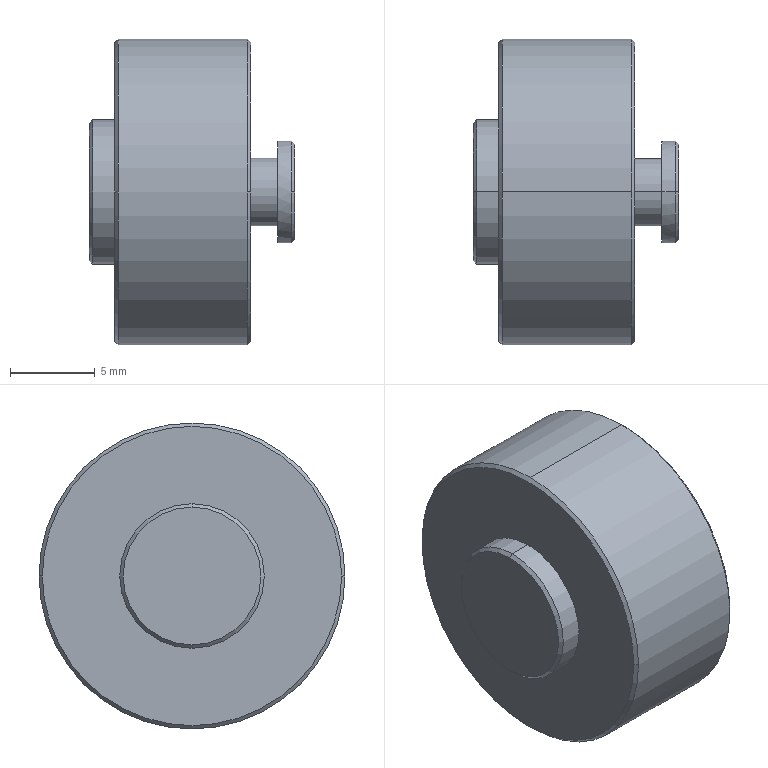Part | STEP file | Guide wheel mechanism revised.sldasm-Part-509 | 1 solid | 22 faces | box 12.1 x 18 x 18 mm | volume 2166 mm3 | cone 9 | cylinder 8 | plane 5 | commonest cylinder face diameters 4 x2 6 x2 8.5 x2 18 x2
STEP:
#1=CARTESIAN_POINT('',(0.,0.,2.));
#2=VERTEX_POINT('',#1);
#3=CARTESIAN_POINT('',(0.,0.,-2.));
#4=VERTEX_POINT('',#3);
#5=CARTESIAN_POINT('',(0.,0.,0.));
#6=DIRECTION('',(-1.,0.,0.));
#7=DIRECTION('',(0.,0.,-1.));
#8=AXIS2_PLACEMENT_3D('',#5,#6,#7);
#9=CIRCLE('',#8,2.);
#10=EDGE_CURVE('',#2,#4,#9,.T.);
#11=ORIENTED_EDGE('',*,*,#10,.F.);
#12=CARTESIAN_POINT('',(1.6,0.,2.));
#13=VERTEX_POINT('',#12);
#14=CARTESIAN_POINT('',(-10.105,0.,2.));
#15=DIRECTION('',(1.,0.,0.));
#16=VECTOR('',#15,1000.);
#17=LINE('',#14,#16);
#18=EDGE_CURVE('',#2,#13,#17,.T.);
#19=ORIENTED_EDGE('',*,*,#18,.T.);
#20=CARTESIAN_POINT('',(1.6,0.,-2.));
#21=VERTEX_POINT('',#20);
#22=CARTESIAN_POINT('',(1.6,0.,0.));
#23=DIRECTION('',(-1.,0.,0.));
#24=DIRECTION('',(0.,0.,-1.));
#25=AXIS2_PLACEMENT_3D('',#22,#23,#24);
#26=CIRCLE('',#25,2.);
#27=EDGE_CURVE('',#13,#21,#26,.T.);
#28=ORIENTED_EDGE('',*,*,#27,.T.);
#29=CARTESIAN_POINT('',(-10.105,0.,-2.));
#30=DIRECTION('',(1.,0.,0.));
#31=VECTOR('',#30,1000.);
#32=LINE('',#29,#31);
#33=EDGE_CURVE('',#4,#21,#32,.T.);
#34=ORIENTED_EDGE('',*,*,#33,.F.);
#35=EDGE_LOOP('',(#11,#19,#28,#34));
#36=FACE_OUTER_BOUND('',#35,.T.);
#37=CARTESIAN_POINT('',(-10.105,0.,0.));
#38=DIRECTION('',(1.,0.,0.));
#39=DIRECTION('',(0.,0.,-1.));
#40=AXIS2_PLACEMENT_3D('',#37,#38,#39);
#41=CYLINDRICAL_SURFACE('',#40,2.);
#42=ADVANCED_FACE('',(#36),#41,.T.);
#43=CARTESIAN_POINT('',(-7.8,9.,0.));
#44=VERTEX_POINT('',#43);
#45=CARTESIAN_POINT('',(-7.8,0.,9.));
#46=VERTEX_POINT('',#45);
#47=CARTESIAN_POINT('',(-7.8,0.,0.));
#48=DIRECTION('',(1.,0.,0.));
#49=DIRECTION('',(0.,0.,-1.));
#50=AXIS2_PLACEMENT_3D('',#47,#48,#49);
#51=CIRCLE('',#50,9.);
#52=EDGE_CURVE('',#44,#46,#51,.T.);
#53=ORIENTED_EDGE('',*,*,#52,.T.);
#54=CARTESIAN_POINT('',(-0.2,0.,9.));
#55=VERTEX_POINT('',#54);
#56=CARTESIAN_POINT('',(-10.105,0.,9.));
#57=DIRECTION('',(1.,0.,0.));
#58=VECTOR('',#57,1000.);
#59=LINE('',#56,#58);
#60=EDGE_CURVE('',#46,#55,#59,.T.);
#61=ORIENTED_EDGE('',*,*,#60,.T.);
#62=CARTESIAN_POINT('',(-0.2,9.,0.));
#63=VERTEX_POINT('',#62);
#64=CARTESIAN_POINT('',(-0.2,0.,0.));
#65=DIRECTION('',(1.,0.,0.));
#66=DIRECTION('',(0.,0.,-1.));
#67=AXIS2_PLACEMENT_3D('',#64,#65,#66);
#68=CIRCLE('',#67,9.);
#69=EDGE_CURVE('',#63,#55,#68,.T.);
#70=ORIENTED_EDGE('',*,*,#69,.F.);
#71=CARTESIAN_POINT('',(-0.2,0.,-9.));
#72=VERTEX_POINT('',#71);
#73=CARTESIAN_POINT('',(-0.2,0.,0.));
#74=DIRECTION('',(1.,0.,0.));
#75=DIRECTION('',(0.,0.,-1.));
#76=AXIS2_PLACEMENT_3D('',#73,#74,#75);
#77=CIRCLE('',#76,9.);
#78=EDGE_CURVE('',#72,#63,#77,.T.);
#79=ORIENTED_EDGE('',*,*,#78,.F.);
#80=CARTESIAN_POINT('',(-7.8,0.,-9.));
#81=VERTEX_POINT('',#80);
#82=CARTESIAN_POINT('',(-10.105,0.,-9.));
#83=DIRECTION('',(1.,0.,0.));
#84=VECTOR('',#83,1000.);
#85=LINE('',#82,#84);
#86=EDGE_CURVE('',#81,#72,#85,.T.);
#87=ORIENTED_EDGE('',*,*,#86,.F.);
#88=CARTESIAN_POINT('',(-7.8,0.,0.));
#89=DIRECTION('',(1.,0.,0.));
#90=DIRECTION('',(0.,0.,-1.));
#91=AXIS2_PLACEMENT_3D('',#88,#89,#90);
#92=CIRCLE('',#91,9.);
#93=EDGE_CURVE('',#81,#44,#92,.T.);
#94=ORIENTED_EDGE('',*,*,#93,.T.);
#95=EDGE_LOOP('',(#53,#61,#70,#79,#87,#94));
#96=FACE_OUTER_BOUND('',#95,.T.);
#97=CARTESIAN_POINT('',(-10.105,0.,0.));
#98=DIRECTION('',(1.,0.,0.));
#99=DIRECTION('',(0.,0.,-1.));
#100=AXIS2_PLACEMENT_3D('',#97,#98,#99);
#101=CYLINDRICAL_SURFACE('',#100,9.);
#102=ADVANCED_FACE('',(#96),#101,.T.);
#103=CARTESIAN_POINT('',(1.6,0.,-3.));
#104=VERTEX_POINT('',#103);
#105=CARTESIAN_POINT('',(1.6,0.,3.));
#106=VERTEX_POINT('',#105);
#107=CARTESIAN_POINT('',(1.6,0.,0.));
#108=DIRECTION('',(1.,0.,0.));
#109=DIRECTION('',(0.,0.,-1.));
#110=AXIS2_PLACEMENT_3D('',#107,#108,#109);
#111=CIRCLE('',#110,3.);
#112=EDGE_CURVE('',#104,#106,#111,.T.);
#113=ORIENTED_EDGE('',*,*,#112,.T.);
#114=CARTESIAN_POINT('',(2.4,0.,3.));
#115=VERTEX_POINT('',#114);
#116=CARTESIAN_POINT('',(-10.105,0.,3.));
#117=DIRECTION('',(1.,0.,0.));
#118=VECTOR('',#117,1000.);
#119=LINE('',#116,#118);
#120=EDGE_CURVE('',#106,#115,#119,.T.);
#121=ORIENTED_EDGE('',*,*,#120,.T.);
#122=CARTESIAN_POINT('',(2.4,3.,0.));
#123=VERTEX_POINT('',#122);
#124=CARTESIAN_POINT('',(2.4,0.,0.));
#125=DIRECTION('',(-1.,0.,0.));
#126=DIRECTION('',(0.,0.,-1.));
#127=AXIS2_PLACEMENT_3D('',#124,#125,#126);
#128=CIRCLE('',#127,3.);
#129=EDGE_CURVE('',#115,#123,#128,.T.);
#130=ORIENTED_EDGE('',*,*,#129,.T.);
#131=CARTESIAN_POINT('',(2.4,0.,-3.));
#132=VERTEX_POINT('',#131);
#133=CARTESIAN_POINT('',(2.4,0.,0.));
#134=DIRECTION('',(-1.,0.,0.));
#135=DIRECTION('',(0.,0.,-1.));
#136=AXIS2_PLACEMENT_3D('',#133,#134,#135);
#137=CIRCLE('',#136,3.);
#138=EDGE_CURVE('',#123,#132,#137,.T.);
#139=ORIENTED_EDGE('',*,*,#138,.T.);
#140=CARTESIAN_POINT('',(-10.105,0.,-3.));
#141=DIRECTION('',(1.,0.,0.));
#142=VECTOR('',#141,1000.);
#143=LINE('',#140,#142);
#144=EDGE_CURVE('',#104,#132,#143,.T.);
#145=ORIENTED_EDGE('',*,*,#144,.F.);
#146=EDGE_LOOP('',(#113,#121,#130,#139,#145));
#147=FACE_OUTER_BOUND('',#146,.T.);
#148=CARTESIAN_POINT('',(-10.105,0.,0.));
#149=DIRECTION('',(1.,0.,0.));
#150=DIRECTION('',(0.,0.,-1.));
#151=AXIS2_PLACEMENT_3D('',#148,#149,#150);
#152=CYLINDRICAL_SURFACE('',#151,3.);
#153=ADVANCED_FACE('',(#147),#152,.T.);
#154=CARTESIAN_POINT('',(2.6,-2.8,0.));
#155=VERTEX_POINT('',#154);
#156=CARTESIAN_POINT('',(2.6,0.,2.8));
#157=VERTEX_POINT('',#156);
#158=CARTESIAN_POINT('',(2.6,0.,0.));
#159=DIRECTION('',(-1.,0.,0.));
#160=DIRECTION('',(0.,0.,1.));
#161=AXIS2_PLACEMENT_3D('',#158,#159,#160);
#162=CIRCLE('',#161,2.8);
#163=EDGE_CURVE('',#155,#157,#162,.T.);
#164=ORIENTED_EDGE('',*,*,#163,.T.);
#165=CARTESIAN_POINT('',(2.4,0.,3.));
#166=DIRECTION('',(-0.7071,0.,0.7071));
#167=VECTOR('',#166,1000.);
#168=LINE('',#165,#167);
#169=EDGE_CURVE('',#157,#115,#168,.T.);
#170=ORIENTED_EDGE('',*,*,#169,.T.);
#171=CARTESIAN_POINT('',(2.4,-3.,0.));
#172=VERTEX_POINT('',#171);
#173=CARTESIAN_POINT('',(2.4,0.,0.));
#174=DIRECTION('',(-1.,0.,0.));
#175=DIRECTION('',(0.,0.,-1.));
#176=AXIS2_PLACEMENT_3D('',#173,#174,#175);
#177=CIRCLE('',#176,3.);
#178=EDGE_CURVE('',#172,#115,#177,.T.);
#179=ORIENTED_EDGE('',*,*,#178,.F.);
#180=CARTESIAN_POINT('',(-498994.601,-499000.,0.000000194));
#181=DIRECTION('',(-0.7071,-0.7071,0.));
#182=VECTOR('',#181,1000.);
#183=LINE('',#180,#182);
#184=EDGE_CURVE('',#155,#172,#183,.T.);
#185=ORIENTED_EDGE('',*,*,#184,.F.);
#186=EDGE_LOOP('',(#164,#170,#179,#185));
#187=FACE_OUTER_BOUND('',#186,.T.);
#188=CARTESIAN_POINT('',(2.4,0.,0.));
#189=DIRECTION('',(-1.,0.,0.));
#190=DIRECTION('',(0.,0.,1.));
#191=AXIS2_PLACEMENT_3D('',#188,#189,#190);
#192=CONICAL_SURFACE('',#191,3.,0.7854);
#193=ADVANCED_FACE('',(#187),#192,.T.);
#194=CARTESIAN_POINT('',(-9.3,0.,-4.25));
#195=VERTEX_POINT('',#194);
#196=CARTESIAN_POINT('',(-9.3,0.,4.25));
#197=VERTEX_POINT('',#196);
#198=CARTESIAN_POINT('',(-9.3,0.,0.));
#199=DIRECTION('',(1.,0.,0.));
#200=DIRECTION('',(0.,0.,-1.));
#201=AXIS2_PLACEMENT_3D('',#198,#199,#200);
#202=CIRCLE('',#201,4.25);
#203=EDGE_CURVE('',#195,#197,#202,.T.);
#204=ORIENTED_EDGE('',*,*,#203,.T.);
#205=CARTESIAN_POINT('',(-8.,0.,4.25));
#206=VERTEX_POINT('',#205);
#207=CARTESIAN_POINT('',(-10.105,0.,4.25));
#208=DIRECTION('',(1.,0.,0.));
#209=VECTOR('',#208,1000.);
#210=LINE('',#207,#209);
#211=EDGE_CURVE('',#197,#206,#210,.T.);
#212=ORIENTED_EDGE('',*,*,#211,.T.);
#213=CARTESIAN_POINT('',(-8.,0.,-4.25));
#214=VERTEX_POINT('',#213);
#215=CARTESIAN_POINT('',(-8.,0.,0.));
#216=DIRECTION('',(-1.,0.,0.));
#217=DIRECTION('',(0.,0.,-1.));
#218=AXIS2_PLACEMENT_3D('',#215,#216,#217);
#219=CIRCLE('',#218,4.25);
#220=EDGE_CURVE('',#206,#214,#219,.T.);
#221=ORIENTED_EDGE('',*,*,#220,.T.);
#222=CARTESIAN_POINT('',(-10.105,0.,-4.25));
#223=DIRECTION('',(1.,0.,0.));
#224=VECTOR('',#223,1000.);
#225=LINE('',#222,#224);
#226=EDGE_CURVE('',#195,#214,#225,.T.);
#227=ORIENTED_EDGE('',*,*,#226,.F.);
#228=EDGE_LOOP('',(#204,#212,#221,#227));
#229=FACE_OUTER_BOUND('',#228,.T.);
#230=CARTESIAN_POINT('',(-10.105,0.,0.));
#231=DIRECTION('',(1.,0.,0.));
#232=DIRECTION('',(0.,0.,-1.));
#233=AXIS2_PLACEMENT_3D('',#230,#231,#232);
#234=CYLINDRICAL_SURFACE('',#233,4.25);
#235=ADVANCED_FACE('',(#229),#234,.T.);
#236=CARTESIAN_POINT('',(-9.5,0.,-4.05));
#237=VERTEX_POINT('',#236);
#238=CARTESIAN_POINT('',(-9.5,0.,4.05));
#239=VERTEX_POINT('',#238);
#240=CARTESIAN_POINT('',(-9.5,0.,0.));
#241=DIRECTION('',(1.,0.,0.));
#242=DIRECTION('',(0.,0.,-1.));
#243=AXIS2_PLACEMENT_3D('',#240,#241,#242);
#244=CIRCLE('',#243,4.05);
#245=EDGE_CURVE('',#237,#239,#244,.T.);
#246=ORIENTED_EDGE('',*,*,#245,.T.);
#247=CARTESIAN_POINT('',(-9.3,0.,4.25));
#248=DIRECTION('',(0.7071,0.,0.7071));
#249=VECTOR('',#248,1000.);
#250=LINE('',#247,#249);
#251=EDGE_CURVE('',#239,#197,#250,.T.);
#252=ORIENTED_EDGE('',*,*,#251,.T.);
#253=ORIENTED_EDGE('',*,*,#203,.F.);
#254=CARTESIAN_POINT('',(-9.3,0.,-4.25));
#255=DIRECTION('',(0.7071,0.,-0.7071));
#256=VECTOR('',#255,1000.);
#257=LINE('',#254,#256);
#258=EDGE_CURVE('',#237,#195,#257,.T.);
#259=ORIENTED_EDGE('',*,*,#258,.F.);
#260=EDGE_LOOP('',(#246,#252,#253,#259));
#261=FACE_OUTER_BOUND('',#260,.T.);
#262=CARTESIAN_POINT('',(-9.3,0.,0.));
#263=DIRECTION('',(1.,0.,0.));
#264=DIRECTION('',(0.,0.,-1.));
#265=AXIS2_PLACEMENT_3D('',#262,#263,#264);
#266=CONICAL_SURFACE('',#265,4.25,0.7854);
#267=ADVANCED_FACE('',(#261),#266,.T.);
#268=CARTESIAN_POINT('',(0.,0.,0.));
#269=DIRECTION('',(-1.,0.,0.));
#270=DIRECTION('',(0.,0.,-1.));
#271=AXIS2_PLACEMENT_3D('',#268,#269,#270);
#272=CIRCLE('',#271,2.);
#273=EDGE_CURVE('',#4,#2,#272,.T.);
#274=ORIENTED_EDGE('',*,*,#273,.T.);
#275=ORIENTED_EDGE('',*,*,#10,.T.);
#276=EDGE_LOOP('',(#274,#275));
#277=FACE_BOUND('',#276,.T.);
#278=CARTESIAN_POINT('',(-0.000000022,8.8,0.));
#279=VERTEX_POINT('',#278);
#280=CARTESIAN_POINT('',(-0.000000022,-8.8,0.));
#281=VERTEX_POINT('',#280);
#282=CARTESIAN_POINT('',(-0.000000022,0.,0.));
#283=DIRECTION('',(1.,0.,0.));
#284=DIRECTION('',(0.,-1.,0.));
#285=AXIS2_PLACEMENT_3D('',#282,#283,#284);
#286=CIRCLE('',#285,8.8);
#287=EDGE_CURVE('',#279,#281,#286,.T.);
#288=ORIENTED_EDGE('',*,*,#287,.T.);
#289=CARTESIAN_POINT('',(-0.000000022,0.,0.));
#290=DIRECTION('',(1.,0.,0.));
#291=DIRECTION('',(0.,0.,1.));
#292=AXIS2_PLACEMENT_3D('',#289,#290,#291);
#293=CIRCLE('',#292,8.8);
#294=EDGE_CURVE('',#281,#279,#293,.T.);
#295=ORIENTED_EDGE('',*,*,#294,.T.);
#296=EDGE_LOOP('',(#288,#295));
#297=FACE_OUTER_BOUND('',#296,.T.);
#298=CARTESIAN_POINT('',(0.,0.,0.));
#299=DIRECTION('',(1.,0.,0.));
#300=DIRECTION('',(0.,0.,-1.));
#301=AXIS2_PLACEMENT_3D('',#298,#299,#300);
#302=PLANE('',#301);
#303=ADVANCED_FACE('',(#277,#297),#302,.T.);
#304=ORIENTED_EDGE('',*,*,#18,.F.);
#305=ORIENTED_EDGE('',*,*,#273,.F.);
#306=ORIENTED_EDGE('',*,*,#33,.T.);
#307=CARTESIAN_POINT('',(1.6,0.,0.));
#308=DIRECTION('',(-1.,0.,0.));
#309=DIRECTION('',(0.,0.,-1.));
#310=AXIS2_PLACEMENT_3D('',#307,#308,#309);
#311=CIRCLE('',#310,2.);
#312=EDGE_CURVE('',#21,#13,#311,.T.);
#313=ORIENTED_EDGE('',*,*,#312,.T.);
#314=EDGE_LOOP('',(#304,#305,#306,#313));
#315=FACE_OUTER_BOUND('',#314,.T.);
#316=CARTESIAN_POINT('',(-10.105,0.,0.));
#317=DIRECTION('',(1.,0.,0.));
#318=DIRECTION('',(0.,0.,-1.));
#319=AXIS2_PLACEMENT_3D('',#316,#317,#318);
#320=CYLINDRICAL_SURFACE('',#319,2.);
#321=ADVANCED_FACE('',(#315),#320,.T.);
#322=CARTESIAN_POINT('',(-0.2,-9.,0.));
#323=VERTEX_POINT('',#322);
#324=CARTESIAN_POINT('',(-498991.203,-499000.,0.000000013));
#325=DIRECTION('',(-0.7071,-0.7071,0.));
#326=VECTOR('',#325,1000.);
#327=LINE('',#324,#326);
#328=EDGE_CURVE('',#281,#323,#327,.T.);
#329=ORIENTED_EDGE('',*,*,#328,.T.);
#330=CARTESIAN_POINT('',(-0.2,0.,0.));
#331=DIRECTION('',(1.,0.,0.));
#332=DIRECTION('',(0.,0.,-1.));
#333=AXIS2_PLACEMENT_3D('',#330,#331,#332);
#334=CIRCLE('',#333,9.);
#335=EDGE_CURVE('',#323,#72,#334,.T.);
#336=ORIENTED_EDGE('',*,*,#335,.T.);
#337=ORIENTED_EDGE('',*,*,#78,.T.);
#338=CARTESIAN_POINT('',(-498991.203,499000.,0.000000012));
#339=DIRECTION('',(0.7071,-0.7071,0.));
#340=VECTOR('',#339,1000.);
#341=LINE('',#338,#340);
#342=EDGE_CURVE('',#63,#279,#341,.T.);
#343=ORIENTED_EDGE('',*,*,#342,.T.);
#344=ORIENTED_EDGE('',*,*,#294,.F.);
#345=EDGE_LOOP('',(#329,#336,#337,#343,#344));
#346=FACE_OUTER_BOUND('',#345,.T.);
#347=CARTESIAN_POINT('',(-0.2,0.,0.));
#348=DIRECTION('',(-1.,0.,0.));
#349=DIRECTION('',(0.,0.,1.));
#350=AXIS2_PLACEMENT_3D('',#347,#348,#349);
#351=CONICAL_SURFACE('',#350,9.,0.7854);
#352=ADVANCED_FACE('',(#346),#351,.T.);
#353=ORIENTED_EDGE('',*,*,#342,.F.);
#354=ORIENTED_EDGE('',*,*,#69,.T.);
#355=CARTESIAN_POINT('',(-0.2,0.,0.));
#356=DIRECTION('',(1.,0.,0.));
#357=DIRECTION('',(0.,0.,-1.));
#358=AXIS2_PLACEMENT_3D('',#355,#356,#357);
#359=CIRCLE('',#358,9.);
#360=EDGE_CURVE('',#55,#323,#359,.T.);
#361=ORIENTED_EDGE('',*,*,#360,.T.);
#362=ORIENTED_EDGE('',*,*,#328,.F.);
#363=ORIENTED_EDGE('',*,*,#287,.F.);
#364=EDGE_LOOP('',(#353,#354,#361,#362,#363));
#365=FACE_OUTER_BOUND('',#364,.T.);
#366=CARTESIAN_POINT('',(-0.2,0.,0.));
#367=DIRECTION('',(-1.,0.,0.));
#368=DIRECTION('',(0.,-1.,0.));
#369=AXIS2_PLACEMENT_3D('',#366,#367,#368);
#370=CONICAL_SURFACE('',#369,9.,0.7854);
#371=ADVANCED_FACE('',(#365),#370,.T.);
#372=ORIENTED_EDGE('',*,*,#312,.F.);
#373=ORIENTED_EDGE('',*,*,#27,.F.);
#374=EDGE_LOOP('',(#372,#373));
#375=FACE_BOUND('',#374,.T.);
#376=ORIENTED_EDGE('',*,*,#112,.F.);
#377=CARTESIAN_POINT('',(1.6,0.,0.));
#378=DIRECTION('',(1.,0.,0.));
#379=DIRECTION('',(0.,0.,-1.));
#380=AXIS2_PLACEMENT_3D('',#377,#378,#379);
#381=CIRCLE('',#380,3.);
#382=EDGE_CURVE('',#106,#104,#381,.T.);
#383=ORIENTED_EDGE('',*,*,#382,.F.);
#384=EDGE_LOOP('',(#376,#383));
#385=FACE_OUTER_BOUND('',#384,.T.);
#386=CARTESIAN_POINT('',(1.6,0.,0.));
#387=DIRECTION('',(1.,0.,0.));
#388=DIRECTION('',(0.,0.,-1.));
#389=AXIS2_PLACEMENT_3D('',#386,#387,#388);
#390=PLANE('',#389);
#391=ADVANCED_FACE('',(#375,#385),#390,.F.);
#392=ORIENTED_EDGE('',*,*,#60,.F.);
#393=CARTESIAN_POINT('',(-7.8,-9.,0.));
#394=VERTEX_POINT('',#393);
#395=CARTESIAN_POINT('',(-7.8,0.,0.));
#396=DIRECTION('',(1.,0.,0.));
#397=DIRECTION('',(0.,0.,-1.));
#398=AXIS2_PLACEMENT_3D('',#395,#396,#397);
#399=CIRCLE('',#398,9.);
#400=EDGE_CURVE('',#46,#394,#399,.T.);
#401=ORIENTED_EDGE('',*,*,#400,.T.);
#402=CARTESIAN_POINT('',(-7.8,0.,0.));
#403=DIRECTION('',(1.,0.,0.));
#404=DIRECTION('',(0.,0.,-1.));
#405=AXIS2_PLACEMENT_3D('',#402,#403,#404);
#406=CIRCLE('',#405,9.);
#407=EDGE_CURVE('',#394,#81,#406,.T.);
#408=ORIENTED_EDGE('',*,*,#407,.T.);
#409=ORIENTED_EDGE('',*,*,#86,.T.);
#410=ORIENTED_EDGE('',*,*,#335,.F.);
#411=ORIENTED_EDGE('',*,*,#360,.F.);
#412=EDGE_LOOP('',(#392,#401,#408,#409,#410,#411));
#413=FACE_OUTER_BOUND('',#412,.T.);
#414=CARTESIAN_POINT('',(-10.105,0.,0.));
#415=DIRECTION('',(1.,0.,0.));
#416=DIRECTION('',(0.,0.,-1.));
#417=AXIS2_PLACEMENT_3D('',#414,#415,#416);
#418=CYLINDRICAL_SURFACE('',#417,9.);
#419=ADVANCED_FACE('',(#413),#418,.T.);
#420=ORIENTED_EDGE('',*,*,#120,.F.);
#421=ORIENTED_EDGE('',*,*,#382,.T.);
#422=ORIENTED_EDGE('',*,*,#144,.T.);
#423=CARTESIAN_POINT('',(2.4,0.,0.));
#424=DIRECTION('',(-1.,0.,0.));
#425=DIRECTION('',(0.,0.,-1.));
#426=AXIS2_PLACEMENT_3D('',#423,#424,#425);
#427=CIRCLE('',#426,3.);
#428=EDGE_CURVE('',#132,#172,#427,.T.);
#429=ORIENTED_EDGE('',*,*,#428,.T.);
#430=ORIENTED_EDGE('',*,*,#178,.T.);
#431=EDGE_LOOP('',(#420,#421,#422,#429,#430));
#432=FACE_OUTER_BOUND('',#431,.T.);
#433=CARTESIAN_POINT('',(-10.105,0.,0.));
#434=DIRECTION('',(1.,0.,0.));
#435=DIRECTION('',(0.,0.,-1.));
#436=AXIS2_PLACEMENT_3D('',#433,#434,#435);
#437=CYLINDRICAL_SURFACE('',#436,3.);
#438=ADVANCED_FACE('',(#432),#437,.T.);
#439=CARTESIAN_POINT('',(-8.,-8.8,0.));
#440=VERTEX_POINT('',#439);
#441=CARTESIAN_POINT('',(498983.202,-499000.,0.000000014));
#442=DIRECTION('',(-0.7071,0.7071,0.));
#443=VECTOR('',#442,1000.);
#444=LINE('',#441,#443);
#445=EDGE_CURVE('',#394,#440,#444,.T.);
#446=ORIENTED_EDGE('',*,*,#445,.T.);
#447=CARTESIAN_POINT('',(-8.,8.8,0.));
#448=VERTEX_POINT('',#447);
#449=CARTESIAN_POINT('',(-8.,0.,0.));
#450=DIRECTION('',(1.,0.,0.));
#451=DIRECTION('',(0.,1.,0.));
#452=AXIS2_PLACEMENT_3D('',#449,#450,#451);
#453=CIRCLE('',#452,8.8);
#454=EDGE_CURVE('',#440,#448,#453,.T.);
#455=ORIENTED_EDGE('',*,*,#454,.T.);
#456=CARTESIAN_POINT('',(498983.202,499000.,0.00000002));
#457=DIRECTION('',(0.7071,0.7071,0.));
#458=VECTOR('',#457,1000.);
#459=LINE('',#456,#458);
#460=EDGE_CURVE('',#448,#44,#459,.T.);
#461=ORIENTED_EDGE('',*,*,#460,.T.);
#462=ORIENTED_EDGE('',*,*,#93,.F.);
#463=ORIENTED_EDGE('',*,*,#407,.F.);
#464=EDGE_LOOP('',(#446,#455,#461,#462,#463));
#465=FACE_OUTER_BOUND('',#464,.T.);
#466=CARTESIAN_POINT('',(-7.8,0.,0.));
#467=DIRECTION('',(1.,0.,0.));
#468=DIRECTION('',(0.,1.,0.));
#469=AXIS2_PLACEMENT_3D('',#466,#467,#468);
#470=CONICAL_SURFACE('',#469,9.,0.7854);
#471=ADVANCED_FACE('',(#465),#470,.T.);
#472=ORIENTED_EDGE('',*,*,#460,.F.);
#473=CARTESIAN_POINT('',(-8.,0.,0.));
#474=DIRECTION('',(1.,0.,0.));
#475=DIRECTION('',(0.,0.,-1.));
#476=AXIS2_PLACEMENT_3D('',#473,#474,#475);
#477=CIRCLE('',#476,8.8);
#478=EDGE_CURVE('',#448,#440,#477,.T.);
#479=ORIENTED_EDGE('',*,*,#478,.T.);
#480=ORIENTED_EDGE('',*,*,#445,.F.);
#481=ORIENTED_EDGE('',*,*,#400,.F.);
#482=ORIENTED_EDGE('',*,*,#52,.F.);
#483=EDGE_LOOP('',(#472,#479,#480,#481,#482));
#484=FACE_OUTER_BOUND('',#483,.T.);
#485=CARTESIAN_POINT('',(-7.8,0.,0.));
#486=DIRECTION('',(1.,0.,0.));
#487=DIRECTION('',(0.,0.,-1.));
#488=AXIS2_PLACEMENT_3D('',#485,#486,#487);
#489=CONICAL_SURFACE('',#488,9.,0.7854);
#490=ADVANCED_FACE('',(#484),#489,.T.);
#491=ORIENTED_EDGE('',*,*,#184,.T.);
#492=ORIENTED_EDGE('',*,*,#428,.F.);
#493=ORIENTED_EDGE('',*,*,#138,.F.);
#494=CARTESIAN_POINT('',(2.6,2.8,0.));
#495=VERTEX_POINT('',#494);
#496=CARTESIAN_POINT('',(-498994.601,499000.,0.000000181));
#497=DIRECTION('',(0.7071,-0.7071,0.));
#498=VECTOR('',#497,1000.);
#499=LINE('',#496,#498);
#500=EDGE_CURVE('',#123,#495,#499,.T.);
#501=ORIENTED_EDGE('',*,*,#500,.T.);
#502=CARTESIAN_POINT('',(2.6,0.,0.));
#503=DIRECTION('',(-1.,0.,0.));
#504=DIRECTION('',(0.,0.,1.));
#505=AXIS2_PLACEMENT_3D('',#502,#503,#504);
#506=CIRCLE('',#505,2.8);
#507=EDGE_CURVE('',#495,#155,#506,.T.);
#508=ORIENTED_EDGE('',*,*,#507,.T.);
#509=EDGE_LOOP('',(#491,#492,#493,#501,#508));
#510=FACE_OUTER_BOUND('',#509,.T.);
#511=CARTESIAN_POINT('',(2.4,0.,0.));
#512=DIRECTION('',(-1.,0.,0.));
#513=DIRECTION('',(0.,0.,1.));
#514=AXIS2_PLACEMENT_3D('',#511,#512,#513);
#515=CONICAL_SURFACE('',#514,3.,0.7854);
#516=ADVANCED_FACE('',(#510),#515,.T.);
#517=ORIENTED_EDGE('',*,*,#169,.F.);
#518=CARTESIAN_POINT('',(2.6,0.,0.));
#519=DIRECTION('',(-1.,0.,0.));
#520=DIRECTION('',(0.,0.,1.));
#521=AXIS2_PLACEMENT_3D('',#518,#519,#520);
#522=CIRCLE('',#521,2.8);
#523=EDGE_CURVE('',#157,#495,#522,.T.);
#524=ORIENTED_EDGE('',*,*,#523,.T.);
#525=ORIENTED_EDGE('',*,*,#500,.F.);
#526=ORIENTED_EDGE('',*,*,#129,.F.);
#527=EDGE_LOOP('',(#517,#524,#525,#526));
#528=FACE_OUTER_BOUND('',#527,.T.);
#529=CARTESIAN_POINT('',(2.4,0.,0.));
#530=DIRECTION('',(-1.,0.,0.));
#531=DIRECTION('',(0.,0.,1.));
#532=AXIS2_PLACEMENT_3D('',#529,#530,#531);
#533=CONICAL_SURFACE('',#532,3.,0.7854);
#534=ADVANCED_FACE('',(#528),#533,.T.);
#535=CARTESIAN_POINT('',(-8.,0.,0.));
#536=DIRECTION('',(-1.,0.,0.));
#537=DIRECTION('',(0.,0.,-1.));
#538=AXIS2_PLACEMENT_3D('',#535,#536,#537);
#539=CIRCLE('',#538,4.25);
#540=EDGE_CURVE('',#214,#206,#539,.T.);
#541=ORIENTED_EDGE('',*,*,#540,.F.);
#542=ORIENTED_EDGE('',*,*,#220,.F.);
#543=EDGE_LOOP('',(#541,#542));
#544=FACE_BOUND('',#543,.T.);
#545=ORIENTED_EDGE('',*,*,#454,.F.);
#546=ORIENTED_EDGE('',*,*,#478,.F.);
#547=EDGE_LOOP('',(#545,#546));
#548=FACE_OUTER_BOUND('',#547,.T.);
#549=CARTESIAN_POINT('',(-8.,0.,0.));
#550=DIRECTION('',(1.,0.,0.));
#551=DIRECTION('',(0.,0.,-1.));
#552=AXIS2_PLACEMENT_3D('',#549,#550,#551);
#553=PLANE('',#552);
#554=ADVANCED_FACE('',(#544,#548),#553,.F.);
#555=ORIENTED_EDGE('',*,*,#163,.F.);
#556=ORIENTED_EDGE('',*,*,#507,.F.);
#557=ORIENTED_EDGE('',*,*,#523,.F.);
#558=EDGE_LOOP('',(#555,#556,#557));
#559=FACE_OUTER_BOUND('',#558,.T.);
#560=CARTESIAN_POINT('',(2.6,0.,0.));
#561=DIRECTION('',(1.,0.,0.));
#562=DIRECTION('',(0.,0.,-1.));
#563=AXIS2_PLACEMENT_3D('',#560,#561,#562);
#564=PLANE('',#563);
#565=ADVANCED_FACE('',(#559),#564,.T.);
#566=ORIENTED_EDGE('',*,*,#211,.F.);
#567=CARTESIAN_POINT('',(-9.3,0.,0.));
#568=DIRECTION('',(1.,0.,0.));
#569=DIRECTION('',(0.,0.,-1.));
#570=AXIS2_PLACEMENT_3D('',#567,#568,#569);
#571=CIRCLE('',#570,4.25);
#572=EDGE_CURVE('',#197,#195,#571,.T.);
#573=ORIENTED_EDGE('',*,*,#572,.T.);
#574=ORIENTED_EDGE('',*,*,#226,.T.);
#575=ORIENTED_EDGE('',*,*,#540,.T.);
#576=EDGE_LOOP('',(#566,#573,#574,#575));
#577=FACE_OUTER_BOUND('',#576,.T.);
#578=CARTESIAN_POINT('',(-10.105,0.,0.));
#579=DIRECTION('',(1.,0.,0.));
#580=DIRECTION('',(0.,0.,-1.));
#581=AXIS2_PLACEMENT_3D('',#578,#579,#580);
#582=CYLINDRICAL_SURFACE('',#581,4.25);
#583=ADVANCED_FACE('',(#577),#582,.T.);
#584=ORIENTED_EDGE('',*,*,#251,.F.);
#585=CARTESIAN_POINT('',(-9.5,0.,0.));
#586=DIRECTION('',(1.,0.,0.));
#587=DIRECTION('',(0.,0.,-1.));
#588=AXIS2_PLACEMENT_3D('',#585,#586,#587);
#589=CIRCLE('',#588,4.05);
#590=EDGE_CURVE('',#239,#237,#589,.T.);
#591=ORIENTED_EDGE('',*,*,#590,.T.);
#592=ORIENTED_EDGE('',*,*,#258,.T.);
#593=ORIENTED_EDGE('',*,*,#572,.F.);
#594=EDGE_LOOP('',(#584,#591,#592,#593));
#595=FACE_OUTER_BOUND('',#594,.T.);
#596=CARTESIAN_POINT('',(-9.3,0.,0.));
#597=DIRECTION('',(1.,0.,0.));
#598=DIRECTION('',(0.,0.,-1.));
#599=AXIS2_PLACEMENT_3D('',#596,#597,#598);
#600=CONICAL_SURFACE('',#599,4.25,0.7854);
#601=ADVANCED_FACE('',(#595),#600,.T.);
#602=ORIENTED_EDGE('',*,*,#245,.F.);
#603=ORIENTED_EDGE('',*,*,#590,.F.);
#604=EDGE_LOOP('',(#602,#603));
#605=FACE_OUTER_BOUND('',#604,.T.);
#606=CARTESIAN_POINT('',(-9.5,0.,0.));
#607=DIRECTION('',(1.,0.,0.));
#608=DIRECTION('',(0.,0.,-1.));
#609=AXIS2_PLACEMENT_3D('',#606,#607,#608);
#610=PLANE('',#609);
#611=ADVANCED_FACE('',(#605),#610,.F.);
#612=CLOSED_SHELL('',(#42,#102,#153,#193,#235,#267,#303,#321,#352,#371,#391,#419,#438,#471,#490,#516,#534,#554,#565,#583,#601,#611));
#613=MANIFOLD_SOLID_BREP('',#612);
#614=CARTESIAN_POINT('',(0.,0.,0.));
#615=DIRECTION('',(0.,0.,1.));
#616=DIRECTION('',(1.,0.,0.));
#617=AXIS2_PLACEMENT_3D('',#614,#615,#616);
#618=(LENGTH_UNIT()NAMED_UNIT(*)SI_UNIT(.MILLI.,.METRE.));
#619=UNCERTAINTY_MEASURE_WITH_UNIT(LENGTH_MEASURE(0.00001),#618,'','');
#620=(NAMED_UNIT(*)PLANE_ANGLE_UNIT()SI_UNIT($,.RADIAN.));
#621=(NAMED_UNIT(*)SI_UNIT($,.STERADIAN.)SOLID_ANGLE_UNIT());
#622=(GEOMETRIC_REPRESENTATION_CONTEXT(3)GLOBAL_UNCERTAINTY_ASSIGNED_CONTEXT((#619))GLOBAL_UNIT_ASSIGNED_CONTEXT((#618,#620,#621))REPRESENTATION_CONTEXT('',''));
#623=ADVANCED_BREP_SHAPE_REPRESENTATION('',(#613,#617),#622);